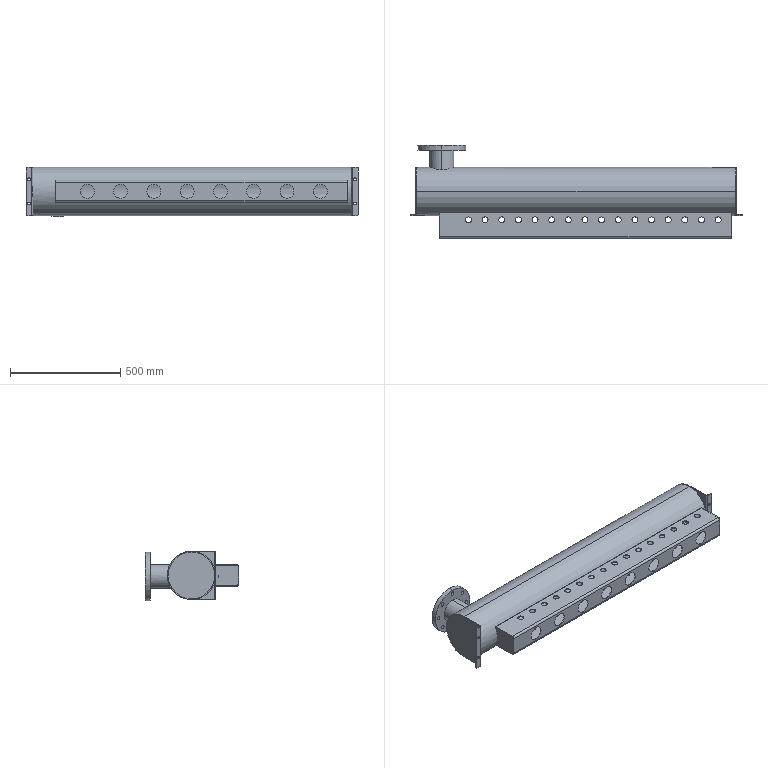Part | SolidWorks | features ICE 14, BaseBody 3, MoveCopyBody 1, MoveFace 1 | 3 solids | 204 faces | box 1506 x 424.041 x 224.313 mm | volume 5157199 mm3 | cylinder 167 | plane 37 | commonest cylinder face diameters 27 x64 18 x16 63 x16 67.2 x16 10.1 x14 12 x12